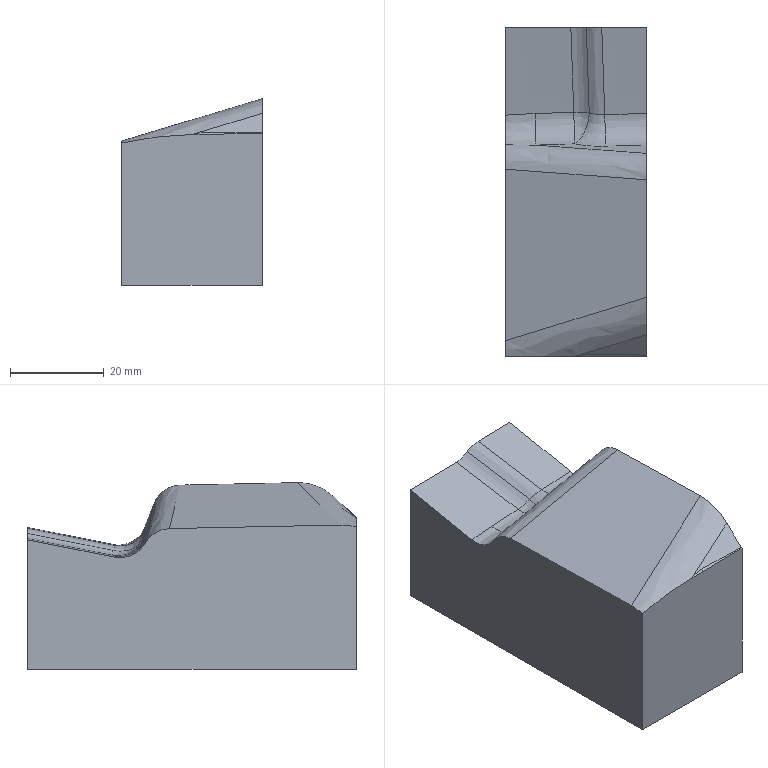Part | NX | features solid 2 | 1 solid | 22 faces | box 30.002 x 70 x 39.765 mm | volume 66479 mm3 | spline 17 | plane 5